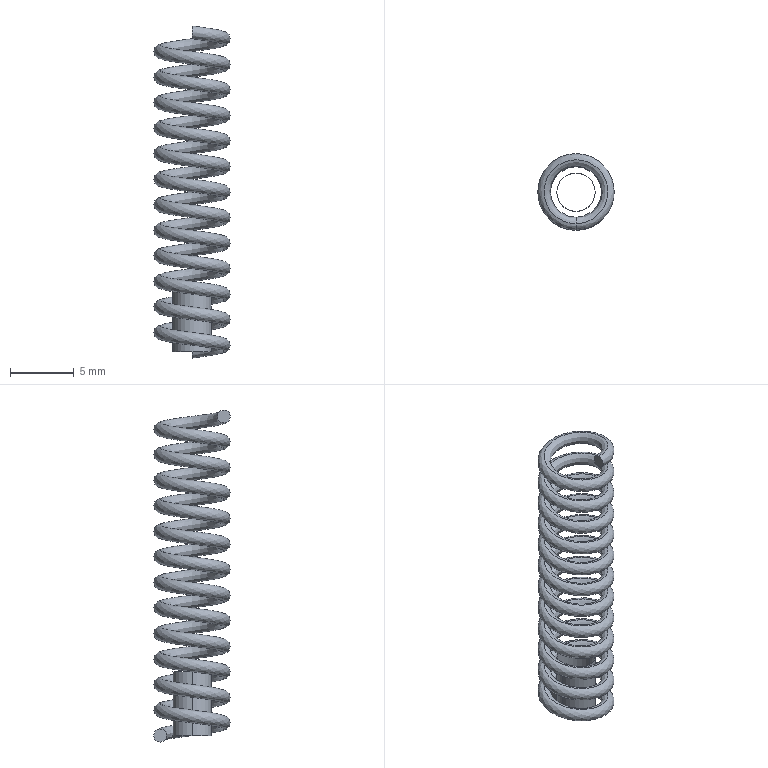Part | NX | features BREP 2 | 1 solid | 6 faces | box 6 x 6 x 26 mm | volume 177.692 mm3 | spline 2 | plane 2 | cylinder 2 | commonest cylinder face diameters 3 x2